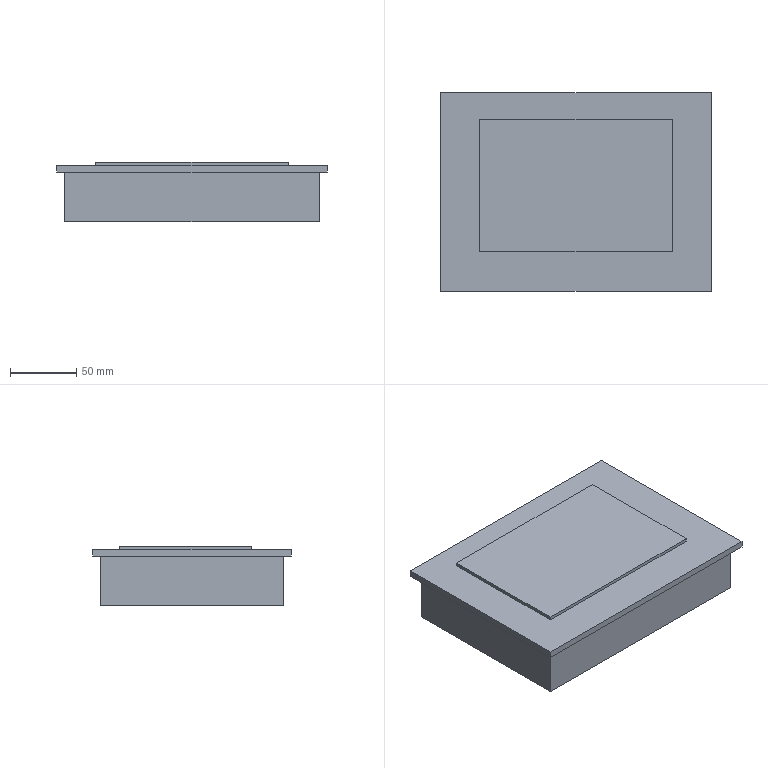Part | STEP file | 7 inch screen | 1 solid | 16 faces | box 204 x 150 x 45 mm | volume 1182850 mm3 | plane 16
STEP:
#1=CARTESIAN_POINT('',(0.,0.,0.));
#2=DIRECTION('',(0.,0.,1.));
#3=DIRECTION('',(1.,0.,0.));
#4=AXIS2_PLACEMENT_3D('',#1,#2,#3);
#5=CARTESIAN_POINT('',(102.,-75.,42.5));
#6=VERTEX_POINT('',#5);
#7=CARTESIAN_POINT('',(102.,75.,42.5));
#8=VERTEX_POINT('',#7);
#9=CARTESIAN_POINT('',(102.,-75.,42.5));
#10=DIRECTION('',(0.,1.,0.));
#11=VECTOR('',#10,1.);
#12=LINE('',#9,#11);
#13=CARTESIAN_POINT('',(0.,0.,42.5));
#14=DIRECTION('',(0.,0.,1.));
#15=DIRECTION('',(1.,0.,0.));
#16=AXIS2_PLACEMENT_3D('',#13,#14,#15);
#17=PLANE('',#16);
#18=CARTESIAN_POINT('',(102.,-75.));
#19=DIRECTION('',(0.,1.));
#20=VECTOR('',#19,1.);
#21=LINE('',#18,#20);
#22=(GEOMETRIC_REPRESENTATION_CONTEXT(2)PARAMETRIC_REPRESENTATION_CONTEXT()REPRESENTATION_CONTEXT('',''));
#23=DEFINITIONAL_REPRESENTATION('',(#21),#22);
#24=PCURVE('',#17,#23);
#25=CARTESIAN_POINT('',(102.,-75.,42.5));
#26=DIRECTION('',(-1.,0.,0.));
#27=DIRECTION('',(0.,0.,1.));
#28=AXIS2_PLACEMENT_3D('',#25,#26,#27);
#29=PLANE('',#28);
#30=CARTESIAN_POINT('',(0.,0.));
#31=DIRECTION('',(0.,1.));
#32=VECTOR('',#31,1.);
#33=LINE('',#30,#32);
#34=(GEOMETRIC_REPRESENTATION_CONTEXT(2)PARAMETRIC_REPRESENTATION_CONTEXT()REPRESENTATION_CONTEXT('',''));
#35=DEFINITIONAL_REPRESENTATION('',(#33),#34);
#36=PCURVE('',#29,#35);
#37=SURFACE_CURVE('',#12,(#24,#36),.PCURVE_S1.);
#38=EDGE_CURVE('',#6,#8,#37,.T.);
#39=ORIENTED_EDGE('',*,*,#38,.T.);
#40=CARTESIAN_POINT('',(-102.,75.,42.5));
#41=VERTEX_POINT('',#40);
#42=CARTESIAN_POINT('',(-102.,75.,42.5));
#43=DIRECTION('',(-1.,0.,0.));
#44=VECTOR('',#43,1.);
#45=LINE('',#42,#44);
#46=CARTESIAN_POINT('',(-102.,75.));
#47=DIRECTION('',(-1.,0.));
#48=VECTOR('',#47,1.);
#49=LINE('',#46,#48);
#50=(GEOMETRIC_REPRESENTATION_CONTEXT(2)PARAMETRIC_REPRESENTATION_CONTEXT()REPRESENTATION_CONTEXT('',''));
#51=DEFINITIONAL_REPRESENTATION('',(#49),#50);
#52=PCURVE('',#17,#51);
#53=CARTESIAN_POINT('',(-102.,75.,42.5));
#54=DIRECTION('',(0.,-1.,0.));
#55=DIRECTION('',(0.,0.,-1.));
#56=AXIS2_PLACEMENT_3D('',#53,#54,#55);
#57=PLANE('',#56);
#58=CARTESIAN_POINT('',(0.,0.));
#59=DIRECTION('',(0.,-1.));
#60=VECTOR('',#59,1.);
#61=LINE('',#58,#60);
#62=(GEOMETRIC_REPRESENTATION_CONTEXT(2)PARAMETRIC_REPRESENTATION_CONTEXT()REPRESENTATION_CONTEXT('',''));
#63=DEFINITIONAL_REPRESENTATION('',(#61),#62);
#64=PCURVE('',#57,#63);
#65=SURFACE_CURVE('',#45,(#52,#64),.PCURVE_S1.);
#66=EDGE_CURVE('',#8,#41,#65,.T.);
#67=ORIENTED_EDGE('',*,*,#66,.T.);
#68=CARTESIAN_POINT('',(-102.,-75.,42.5));
#69=VERTEX_POINT('',#68);
#70=CARTESIAN_POINT('',(-102.,-75.,42.5));
#71=DIRECTION('',(0.,-1.,0.));
#72=VECTOR('',#71,1.);
#73=LINE('',#70,#72);
#74=CARTESIAN_POINT('',(-102.,-75.));
#75=DIRECTION('',(0.,-1.));
#76=VECTOR('',#75,1.);
#77=LINE('',#74,#76);
#78=(GEOMETRIC_REPRESENTATION_CONTEXT(2)PARAMETRIC_REPRESENTATION_CONTEXT()REPRESENTATION_CONTEXT('',''));
#79=DEFINITIONAL_REPRESENTATION('',(#77),#78);
#80=PCURVE('',#17,#79);
#81=CARTESIAN_POINT('',(-102.,-75.,42.5));
#82=DIRECTION('',(1.,0.,0.));
#83=DIRECTION('',(0.,0.,-1.));
#84=AXIS2_PLACEMENT_3D('',#81,#82,#83);
#85=PLANE('',#84);
#86=CARTESIAN_POINT('',(0.,0.));
#87=DIRECTION('',(0.,-1.));
#88=VECTOR('',#87,1.);
#89=LINE('',#86,#88);
#90=(GEOMETRIC_REPRESENTATION_CONTEXT(2)PARAMETRIC_REPRESENTATION_CONTEXT()REPRESENTATION_CONTEXT('',''));
#91=DEFINITIONAL_REPRESENTATION('',(#89),#90);
#92=PCURVE('',#85,#91);
#93=SURFACE_CURVE('',#73,(#80,#92),.PCURVE_S1.);
#94=EDGE_CURVE('',#41,#69,#93,.T.);
#95=ORIENTED_EDGE('',*,*,#94,.T.);
#96=CARTESIAN_POINT('',(-102.,-75.,42.5));
#97=DIRECTION('',(1.,0.,0.));
#98=VECTOR('',#97,1.);
#99=LINE('',#96,#98);
#100=CARTESIAN_POINT('',(-102.,-75.));
#101=DIRECTION('',(1.,0.));
#102=VECTOR('',#101,1.);
#103=LINE('',#100,#102);
#104=(GEOMETRIC_REPRESENTATION_CONTEXT(2)PARAMETRIC_REPRESENTATION_CONTEXT()REPRESENTATION_CONTEXT('',''));
#105=DEFINITIONAL_REPRESENTATION('',(#103),#104);
#106=PCURVE('',#17,#105);
#107=CARTESIAN_POINT('',(-102.,-75.,42.5));
#108=DIRECTION('',(0.,1.,0.));
#109=DIRECTION('',(0.,0.,1.));
#110=AXIS2_PLACEMENT_3D('',#107,#108,#109);
#111=PLANE('',#110);
#112=CARTESIAN_POINT('',(0.,0.));
#113=DIRECTION('',(0.,1.));
#114=VECTOR('',#113,1.);
#115=LINE('',#112,#114);
#116=(GEOMETRIC_REPRESENTATION_CONTEXT(2)PARAMETRIC_REPRESENTATION_CONTEXT()REPRESENTATION_CONTEXT('',''));
#117=DEFINITIONAL_REPRESENTATION('',(#115),#116);
#118=PCURVE('',#111,#117);
#119=SURFACE_CURVE('',#99,(#106,#118),.PCURVE_S1.);
#120=EDGE_CURVE('',#69,#6,#119,.T.);
#121=ORIENTED_EDGE('',*,*,#120,.T.);
#122=EDGE_LOOP('',(#39,#67,#95,#121));
#123=FACE_BOUND('',#122,.T.);
#124=CARTESIAN_POINT('',(72.5,-45.,42.5));
#125=VERTEX_POINT('',#124);
#126=CARTESIAN_POINT('',(-72.5,-45.,42.5));
#127=VERTEX_POINT('',#126);
#128=CARTESIAN_POINT('',(0.,-45.,42.5));
#129=DIRECTION('',(-1.,0.,0.));
#130=VECTOR('',#129,1.);
#131=LINE('',#128,#130);
#132=CARTESIAN_POINT('',(0.,-45.));
#133=DIRECTION('',(-1.,0.));
#134=VECTOR('',#133,1.);
#135=LINE('',#132,#134);
#136=(GEOMETRIC_REPRESENTATION_CONTEXT(2)PARAMETRIC_REPRESENTATION_CONTEXT()REPRESENTATION_CONTEXT('',''));
#137=DEFINITIONAL_REPRESENTATION('',(#135),#136);
#138=PCURVE('',#17,#137);
#139=CARTESIAN_POINT('',(-72.5,-45.,45.));
#140=DIRECTION('',(0.,1.,0.));
#141=DIRECTION('',(-1.,0.,0.));
#142=AXIS2_PLACEMENT_3D('',#139,#140,#141);
#143=PLANE('',#142);
#144=CARTESIAN_POINT('',(-72.5,-2.5));
#145=DIRECTION('',(1.,0.));
#146=VECTOR('',#145,1.);
#147=LINE('',#144,#146);
#148=(GEOMETRIC_REPRESENTATION_CONTEXT(2)PARAMETRIC_REPRESENTATION_CONTEXT()REPRESENTATION_CONTEXT('',''));
#149=DEFINITIONAL_REPRESENTATION('',(#147),#148);
#150=PCURVE('',#143,#149);
#151=SURFACE_CURVE('',#131,(#138,#150),.PCURVE_S1.);
#152=EDGE_CURVE('',#125,#127,#151,.T.);
#153=ORIENTED_EDGE('',*,*,#152,.T.);
#154=CARTESIAN_POINT('',(-72.5,55.,42.5));
#155=VERTEX_POINT('',#154);
#156=CARTESIAN_POINT('',(-72.5,0.,42.5));
#157=DIRECTION('',(0.,1.,0.));
#158=VECTOR('',#157,1.);
#159=LINE('',#156,#158);
#160=CARTESIAN_POINT('',(-72.5,0.));
#161=DIRECTION('',(0.,1.));
#162=VECTOR('',#161,1.);
#163=LINE('',#160,#162);
#164=(GEOMETRIC_REPRESENTATION_CONTEXT(2)PARAMETRIC_REPRESENTATION_CONTEXT()REPRESENTATION_CONTEXT('',''));
#165=DEFINITIONAL_REPRESENTATION('',(#163),#164);
#166=PCURVE('',#17,#165);
#167=CARTESIAN_POINT('',(-72.5,55.,45.));
#168=DIRECTION('',(1.,0.,0.));
#169=DIRECTION('',(0.,0.,-1.));
#170=AXIS2_PLACEMENT_3D('',#167,#168,#169);
#171=PLANE('',#170);
#172=CARTESIAN_POINT('',(2.5,-55.));
#173=DIRECTION('',(0.,1.));
#174=VECTOR('',#173,1.);
#175=LINE('',#172,#174);
#176=(GEOMETRIC_REPRESENTATION_CONTEXT(2)PARAMETRIC_REPRESENTATION_CONTEXT()REPRESENTATION_CONTEXT('',''));
#177=DEFINITIONAL_REPRESENTATION('',(#175),#176);
#178=PCURVE('',#171,#177);
#179=SURFACE_CURVE('',#159,(#166,#178),.PCURVE_S1.);
#180=EDGE_CURVE('',#127,#155,#179,.T.);
#181=ORIENTED_EDGE('',*,*,#180,.T.);
#182=CARTESIAN_POINT('',(72.5,55.,42.5));
#183=VERTEX_POINT('',#182);
#184=CARTESIAN_POINT('',(0.,55.,42.5));
#185=DIRECTION('',(1.,0.,0.));
#186=VECTOR('',#185,1.);
#187=LINE('',#184,#186);
#188=CARTESIAN_POINT('',(0.,55.));
#189=DIRECTION('',(1.,0.));
#190=VECTOR('',#189,1.);
#191=LINE('',#188,#190);
#192=(GEOMETRIC_REPRESENTATION_CONTEXT(2)PARAMETRIC_REPRESENTATION_CONTEXT()REPRESENTATION_CONTEXT('',''));
#193=DEFINITIONAL_REPRESENTATION('',(#191),#192);
#194=PCURVE('',#17,#193);
#195=CARTESIAN_POINT('',(-72.5,55.,45.));
#196=DIRECTION('',(0.,-1.,0.));
#197=DIRECTION('',(1.,0.,0.));
#198=AXIS2_PLACEMENT_3D('',#195,#196,#197);
#199=PLANE('',#198);
#200=CARTESIAN_POINT('',(72.5,-2.5));
#201=DIRECTION('',(1.,0.));
#202=VECTOR('',#201,1.);
#203=LINE('',#200,#202);
#204=(GEOMETRIC_REPRESENTATION_CONTEXT(2)PARAMETRIC_REPRESENTATION_CONTEXT()REPRESENTATION_CONTEXT('',''));
#205=DEFINITIONAL_REPRESENTATION('',(#203),#204);
#206=PCURVE('',#199,#205);
#207=SURFACE_CURVE('',#187,(#194,#206),.PCURVE_S1.);
#208=EDGE_CURVE('',#155,#183,#207,.T.);
#209=ORIENTED_EDGE('',*,*,#208,.T.);
#210=CARTESIAN_POINT('',(72.5,0.,42.5));
#211=DIRECTION('',(0.,-1.,0.));
#212=VECTOR('',#211,1.);
#213=LINE('',#210,#212);
#214=CARTESIAN_POINT('',(72.5,0.));
#215=DIRECTION('',(0.,-1.));
#216=VECTOR('',#215,1.);
#217=LINE('',#214,#216);
#218=(GEOMETRIC_REPRESENTATION_CONTEXT(2)PARAMETRIC_REPRESENTATION_CONTEXT()REPRESENTATION_CONTEXT('',''));
#219=DEFINITIONAL_REPRESENTATION('',(#217),#218);
#220=PCURVE('',#17,#219);
#221=CARTESIAN_POINT('',(72.5,55.,45.));
#222=DIRECTION('',(-1.,0.,0.));
#223=DIRECTION('',(0.,-1.,0.));
#224=AXIS2_PLACEMENT_3D('',#221,#222,#223);
#225=PLANE('',#224);
#226=CARTESIAN_POINT('',(55.,-2.5));
#227=DIRECTION('',(1.,0.));
#228=VECTOR('',#227,1.);
#229=LINE('',#226,#228);
#230=(GEOMETRIC_REPRESENTATION_CONTEXT(2)PARAMETRIC_REPRESENTATION_CONTEXT()REPRESENTATION_CONTEXT('',''));
#231=DEFINITIONAL_REPRESENTATION('',(#229),#230);
#232=PCURVE('',#225,#231);
#233=SURFACE_CURVE('',#213,(#220,#232),.PCURVE_S1.);
#234=EDGE_CURVE('',#183,#125,#233,.T.);
#235=ORIENTED_EDGE('',*,*,#234,.T.);
#236=EDGE_LOOP('',(#153,#181,#209,#235));
#237=FACE_BOUND('',#236,.T.);
#238=ADVANCED_FACE('',(#123,#237),#17,.T.);
#239=CARTESIAN_POINT('',(96.,-69.,37.5));
#240=VERTEX_POINT('',#239);
#241=CARTESIAN_POINT('',(96.,69.,37.5));
#242=VERTEX_POINT('',#241);
#243=CARTESIAN_POINT('',(96.,-69.,37.5));
#244=DIRECTION('',(0.,1.,0.));
#245=VECTOR('',#244,1.);
#246=LINE('',#243,#245);
#247=CARTESIAN_POINT('',(96.,-69.,40.));
#248=DIRECTION('',(-1.,0.,0.));
#249=DIRECTION('',(0.,0.,1.));
#250=AXIS2_PLACEMENT_3D('',#247,#248,#249);
#251=PLANE('',#250);
#252=CARTESIAN_POINT('',(-2.5,0.));
#253=DIRECTION('',(0.,1.));
#254=VECTOR('',#253,1.);
#255=LINE('',#252,#254);
#256=(GEOMETRIC_REPRESENTATION_CONTEXT(2)PARAMETRIC_REPRESENTATION_CONTEXT()REPRESENTATION_CONTEXT('',''));
#257=DEFINITIONAL_REPRESENTATION('',(#255),#256);
#258=PCURVE('',#251,#257);
#259=CARTESIAN_POINT('',(0.,0.,37.5));
#260=DIRECTION('',(0.,0.,1.));
#261=DIRECTION('',(1.,0.,0.));
#262=AXIS2_PLACEMENT_3D('',#259,#260,#261);
#263=PLANE('',#262);
#264=CARTESIAN_POINT('',(96.,-69.));
#265=DIRECTION('',(0.,1.));
#266=VECTOR('',#265,1.);
#267=LINE('',#264,#266);
#268=(GEOMETRIC_REPRESENTATION_CONTEXT(2)PARAMETRIC_REPRESENTATION_CONTEXT()REPRESENTATION_CONTEXT('',''));
#269=DEFINITIONAL_REPRESENTATION('',(#267),#268);
#270=PCURVE('',#263,#269);
#271=SURFACE_CURVE('',#246,(#258,#270),.PCURVE_S1.);
#272=EDGE_CURVE('',#240,#242,#271,.T.);
#273=ORIENTED_EDGE('',*,*,#272,.F.);
#274=CARTESIAN_POINT('',(96.,-69.,0.));
#275=VERTEX_POINT('',#274);
#276=CARTESIAN_POINT('',(96.,-69.,40.));
#277=DIRECTION('',(0.,0.,-1.));
#278=VECTOR('',#277,1.);
#279=LINE('',#276,#278);
#280=CARTESIAN_POINT('',(0.,0.));
#281=DIRECTION('',(-1.,0.));
#282=VECTOR('',#281,1.);
#283=LINE('',#280,#282);
#284=(GEOMETRIC_REPRESENTATION_CONTEXT(2)PARAMETRIC_REPRESENTATION_CONTEXT()REPRESENTATION_CONTEXT('',''));
#285=DEFINITIONAL_REPRESENTATION('',(#283),#284);
#286=PCURVE('',#251,#285);
#287=CARTESIAN_POINT('',(-96.,-69.,40.));
#288=DIRECTION('',(0.,1.,0.));
#289=DIRECTION('',(0.,0.,1.));
#290=AXIS2_PLACEMENT_3D('',#287,#288,#289);
#291=PLANE('',#290);
#292=CARTESIAN_POINT('',(0.,192.));
#293=DIRECTION('',(-1.,0.));
#294=VECTOR('',#293,1.);
#295=LINE('',#292,#294);
#296=(GEOMETRIC_REPRESENTATION_CONTEXT(2)PARAMETRIC_REPRESENTATION_CONTEXT()REPRESENTATION_CONTEXT('',''));
#297=DEFINITIONAL_REPRESENTATION('',(#295),#296);
#298=PCURVE('',#291,#297);
#299=SURFACE_CURVE('',#279,(#286,#298),.PCURVE_S1.);
#300=EDGE_CURVE('',#240,#275,#299,.T.);
#301=ORIENTED_EDGE('',*,*,#300,.T.);
#302=CARTESIAN_POINT('',(96.,69.,0.));
#303=VERTEX_POINT('',#302);
#304=CARTESIAN_POINT('',(96.,-69.,0.));
#305=DIRECTION('',(0.,1.,0.));
#306=VECTOR('',#305,1.);
#307=LINE('',#304,#306);
#308=CARTESIAN_POINT('',(-40.,0.));
#309=DIRECTION('',(0.,1.));
#310=VECTOR('',#309,1.);
#311=LINE('',#308,#310);
#312=(GEOMETRIC_REPRESENTATION_CONTEXT(2)PARAMETRIC_REPRESENTATION_CONTEXT()REPRESENTATION_CONTEXT('',''));
#313=DEFINITIONAL_REPRESENTATION('',(#311),#312);
#314=PCURVE('',#251,#313);
#315=CARTESIAN_POINT('',(0.,0.,0.));
#316=DIRECTION('',(0.,0.,-1.));
#317=DIRECTION('',(-1.,0.,0.));
#318=AXIS2_PLACEMENT_3D('',#315,#316,#317);
#319=PLANE('',#318);
#320=CARTESIAN_POINT('',(-96.,-69.));
#321=DIRECTION('',(0.,1.));
#322=VECTOR('',#321,1.);
#323=LINE('',#320,#322);
#324=(GEOMETRIC_REPRESENTATION_CONTEXT(2)PARAMETRIC_REPRESENTATION_CONTEXT()REPRESENTATION_CONTEXT('',''));
#325=DEFINITIONAL_REPRESENTATION('',(#323),#324);
#326=PCURVE('',#319,#325);
#327=SURFACE_CURVE('',#307,(#314,#326),.PCURVE_S1.);
#328=EDGE_CURVE('',#275,#303,#327,.T.);
#329=ORIENTED_EDGE('',*,*,#328,.T.);
#330=CARTESIAN_POINT('',(96.,69.,40.));
#331=DIRECTION('',(0.,0.,-1.));
#332=VECTOR('',#331,1.);
#333=LINE('',#330,#332);
#334=CARTESIAN_POINT('',(0.,138.));
#335=DIRECTION('',(-1.,0.));
#336=VECTOR('',#335,1.);
#337=LINE('',#334,#336);
#338=(GEOMETRIC_REPRESENTATION_CONTEXT(2)PARAMETRIC_REPRESENTATION_CONTEXT()REPRESENTATION_CONTEXT('',''));
#339=DEFINITIONAL_REPRESENTATION('',(#337),#338);
#340=PCURVE('',#251,#339);
#341=CARTESIAN_POINT('',(-96.,69.,40.));
#342=DIRECTION('',(0.,-1.,0.));
#343=DIRECTION('',(0.,0.,-1.));
#344=AXIS2_PLACEMENT_3D('',#341,#342,#343);
#345=PLANE('',#344);
#346=CARTESIAN_POINT('',(0.,192.));
#347=DIRECTION('',(1.,0.));
#348=VECTOR('',#347,1.);
#349=LINE('',#346,#348);
#350=(GEOMETRIC_REPRESENTATION_CONTEXT(2)PARAMETRIC_REPRESENTATION_CONTEXT()REPRESENTATION_CONTEXT('',''));
#351=DEFINITIONAL_REPRESENTATION('',(#349),#350);
#352=PCURVE('',#345,#351);
#353=SURFACE_CURVE('',#333,(#340,#352),.PCURVE_S1.);
#354=EDGE_CURVE('',#242,#303,#353,.T.);
#355=ORIENTED_EDGE('',*,*,#354,.F.);
#356=EDGE_LOOP('',(#273,#301,#329,#355));
#357=FACE_BOUND('',#356,.T.);
#358=ADVANCED_FACE('',(#357),#251,.F.);
#359=CARTESIAN_POINT('',(-96.,69.,37.5));
#360=VERTEX_POINT('',#359);
#361=CARTESIAN_POINT('',(-96.,69.,37.5));
#362=DIRECTION('',(-1.,0.,0.));
#363=VECTOR('',#362,1.);
#364=LINE('',#361,#363);
#365=CARTESIAN_POINT('',(2.5,0.));
#366=DIRECTION('',(0.,-1.));
#367=VECTOR('',#366,1.);
#368=LINE('',#365,#367);
#369=(GEOMETRIC_REPRESENTATION_CONTEXT(2)PARAMETRIC_REPRESENTATION_CONTEXT()REPRESENTATION_CONTEXT('',''));
#370=DEFINITIONAL_REPRESENTATION('',(#368),#369);
#371=PCURVE('',#345,#370);
#372=CARTESIAN_POINT('',(-96.,69.));
#373=DIRECTION('',(-1.,0.));
#374=VECTOR('',#373,1.);
#375=LINE('',#372,#374);
#376=(GEOMETRIC_REPRESENTATION_CONTEXT(2)PARAMETRIC_REPRESENTATION_CONTEXT()REPRESENTATION_CONTEXT('',''));
#377=DEFINITIONAL_REPRESENTATION('',(#375),#376);
#378=PCURVE('',#263,#377);
#379=SURFACE_CURVE('',#364,(#371,#378),.PCURVE_S1.);
#380=EDGE_CURVE('',#242,#360,#379,.T.);
#381=ORIENTED_EDGE('',*,*,#380,.F.);
#382=ORIENTED_EDGE('',*,*,#354,.T.);
#383=CARTESIAN_POINT('',(-96.,69.,0.));
#384=VERTEX_POINT('',#383);
#385=CARTESIAN_POINT('',(-96.,69.,0.));
#386=DIRECTION('',(-1.,0.,0.));
#387=VECTOR('',#386,1.);
#388=LINE('',#385,#387);
#389=CARTESIAN_POINT('',(40.,0.));
#390=DIRECTION('',(0.,-1.));
#391=VECTOR('',#390,1.);
#392=LINE('',#389,#391);
#393=(GEOMETRIC_REPRESENTATION_CONTEXT(2)PARAMETRIC_REPRESENTATION_CONTEXT()REPRESENTATION_CONTEXT('',''));
#394=DEFINITIONAL_REPRESENTATION('',(#392),#393);
#395=PCURVE('',#345,#394);
#396=CARTESIAN_POINT('',(96.,69.));
#397=DIRECTION('',(1.,0.));
#398=VECTOR('',#397,1.);
#399=LINE('',#396,#398);
#400=(GEOMETRIC_REPRESENTATION_CONTEXT(2)PARAMETRIC_REPRESENTATION_CONTEXT()REPRESENTATION_CONTEXT('',''));
#401=DEFINITIONAL_REPRESENTATION('',(#399),#400);
#402=PCURVE('',#319,#401);
#403=SURFACE_CURVE('',#388,(#395,#402),.PCURVE_S1.);
#404=EDGE_CURVE('',#303,#384,#403,.T.);
#405=ORIENTED_EDGE('',*,*,#404,.T.);
#406=CARTESIAN_POINT('',(-96.,69.,40.));
#407=DIRECTION('',(0.,0.,-1.));
#408=VECTOR('',#407,1.);
#409=LINE('',#406,#408);
#410=CARTESIAN_POINT('',(0.,0.));
#411=DIRECTION('',(1.,0.));
#412=VECTOR('',#411,1.);
#413=LINE('',#410,#412);
#414=(GEOMETRIC_REPRESENTATION_CONTEXT(2)PARAMETRIC_REPRESENTATION_CONTEXT()REPRESENTATION_CONTEXT('',''));
#415=DEFINITIONAL_REPRESENTATION('',(#413),#414);
#416=PCURVE('',#345,#415);
#417=CARTESIAN_POINT('',(-96.,-69.,40.));
#418=DIRECTION('',(1.,0.,0.));
#419=DIRECTION('',(0.,0.,-1.));
#420=AXIS2_PLACEMENT_3D('',#417,#418,#419);
#421=PLANE('',#420);
#422=CARTESIAN_POINT('',(0.,138.));
#423=DIRECTION('',(1.,0.));
#424=VECTOR('',#423,1.);
#425=LINE('',#422,#424);
#426=(GEOMETRIC_REPRESENTATION_CONTEXT(2)PARAMETRIC_REPRESENTATION_CONTEXT()REPRESENTATION_CONTEXT('',''));
#427=DEFINITIONAL_REPRESENTATION('',(#425),#426);
#428=PCURVE('',#421,#427);
#429=SURFACE_CURVE('',#409,(#416,#428),.PCURVE_S1.);
#430=EDGE_CURVE('',#360,#384,#429,.T.);
#431=ORIENTED_EDGE('',*,*,#430,.F.);
#432=EDGE_LOOP('',(#381,#382,#405,#431));
#433=FACE_BOUND('',#432,.T.);
#434=ADVANCED_FACE('',(#433),#345,.F.);
#435=CARTESIAN_POINT('',(-96.,-69.,37.5));
#436=VERTEX_POINT('',#435);
#437=CARTESIAN_POINT('',(-96.,-69.,37.5));
#438=DIRECTION('',(0.,-1.,0.));
#439=VECTOR('',#438,1.);
#440=LINE('',#437,#439);
#441=CARTESIAN_POINT('',(2.5,0.));
#442=DIRECTION('',(0.,-1.));
#443=VECTOR('',#442,1.);
#444=LINE('',#441,#443);
#445=(GEOMETRIC_REPRESENTATION_CONTEXT(2)PARAMETRIC_REPRESENTATION_CONTEXT()REPRESENTATION_CONTEXT('',''));
#446=DEFINITIONAL_REPRESENTATION('',(#444),#445);
#447=PCURVE('',#421,#446);
#448=CARTESIAN_POINT('',(-96.,-69.));
#449=DIRECTION('',(0.,-1.));
#450=VECTOR('',#449,1.);
#451=LINE('',#448,#450);
#452=(GEOMETRIC_REPRESENTATION_CONTEXT(2)PARAMETRIC_REPRESENTATION_CONTEXT()REPRESENTATION_CONTEXT('',''));
#453=DEFINITIONAL_REPRESENTATION('',(#451),#452);
#454=PCURVE('',#263,#453);
#455=SURFACE_CURVE('',#440,(#447,#454),.PCURVE_S1.);
#456=EDGE_CURVE('',#360,#436,#455,.T.);
#457=ORIENTED_EDGE('',*,*,#456,.F.);
#458=ORIENTED_EDGE('',*,*,#430,.T.);
#459=CARTESIAN_POINT('',(-96.,-69.,0.));
#460=VERTEX_POINT('',#459);
#461=CARTESIAN_POINT('',(-96.,-69.,0.));
#462=DIRECTION('',(0.,-1.,0.));
#463=VECTOR('',#462,1.);
#464=LINE('',#461,#463);
#465=CARTESIAN_POINT('',(40.,0.));
#466=DIRECTION('',(0.,-1.));
#467=VECTOR('',#466,1.);
#468=LINE('',#465,#467);
#469=(GEOMETRIC_REPRESENTATION_CONTEXT(2)PARAMETRIC_REPRESENTATION_CONTEXT()REPRESENTATION_CONTEXT('',''));
#470=DEFINITIONAL_REPRESENTATION('',(#468),#469);
#471=PCURVE('',#421,#470);
#472=CARTESIAN_POINT('',(96.,-69.));
#473=DIRECTION('',(0.,-1.));
#474=VECTOR('',#473,1.);
#475=LINE('',#472,#474);
#476=(GEOMETRIC_REPRESENTATION_CONTEXT(2)PARAMETRIC_REPRESENTATION_CONTEXT()REPRESENTATION_CONTEXT('',''));
#477=DEFINITIONAL_REPRESENTATION('',(#475),#476);
#478=PCURVE('',#319,#477);
#479=SURFACE_CURVE('',#464,(#471,#478),.PCURVE_S1.);
#480=EDGE_CURVE('',#384,#460,#479,.T.);
#481=ORIENTED_EDGE('',*,*,#480,.T.);
#482=CARTESIAN_POINT('',(-96.,-69.,40.));
#483=DIRECTION('',(0.,0.,-1.));
#484=VECTOR('',#483,1.);
#485=LINE('',#482,#484);
#486=CARTESIAN_POINT('',(0.,0.));
#487=DIRECTION('',(1.,0.));
#488=VECTOR('',#487,1.);
#489=LINE('',#486,#488);
#490=(GEOMETRIC_REPRESENTATION_CONTEXT(2)PARAMETRIC_REPRESENTATION_CONTEXT()REPRESENTATION_CONTEXT('',''));
#491=DEFINITIONAL_REPRESENTATION('',(#489),#490);
#492=PCURVE('',#421,#491);
#493=CARTESIAN_POINT('',(0.,0.));
#494=DIRECTION('',(-1.,0.));
#495=VECTOR('',#494,1.);
#496=LINE('',#493,#495);
#497=(GEOMETRIC_REPRESENTATION_CONTEXT(2)PARAMETRIC_REPRESENTATION_CONTEXT()REPRESENTATION_CONTEXT('',''));
#498=DEFINITIONAL_REPRESENTATION('',(#496),#497);
#499=PCURVE('',#291,#498);
#500=SURFACE_CURVE('',#485,(#492,#499),.PCURVE_S1.);
#501=EDGE_CURVE('',#436,#460,#500,.T.);
#502=ORIENTED_EDGE('',*,*,#501,.F.);
#503=EDGE_LOOP('',(#457,#458,#481,#502));
#504=FACE_BOUND('',#503,.T.);
#505=ADVANCED_FACE('',(#504),#421,.F.);
#506=CARTESIAN_POINT('',(-96.,-69.,37.5));
#507=DIRECTION('',(1.,0.,0.));
#508=VECTOR('',#507,1.);
#509=LINE('',#506,#508);
#510=CARTESIAN_POINT('',(-2.5,0.));
#511=DIRECTION('',(0.,1.));
#512=VECTOR('',#511,1.);
#513=LINE('',#510,#512);
#514=(GEOMETRIC_REPRESENTATION_CONTEXT(2)PARAMETRIC_REPRESENTATION_CONTEXT()REPRESENTATION_CONTEXT('',''));
#515=DEFINITIONAL_REPRESENTATION('',(#513),#514);
#516=PCURVE('',#291,#515);
#517=CARTESIAN_POINT('',(-96.,-69.));
#518=DIRECTION('',(1.,0.));
#519=VECTOR('',#518,1.);
#520=LINE('',#517,#519);
#521=(GEOMETRIC_REPRESENTATION_CONTEXT(2)PARAMETRIC_REPRESENTATION_CONTEXT()REPRESENTATION_CONTEXT('',''));
#522=DEFINITIONAL_REPRESENTATION('',(#520),#521);
#523=PCURVE('',#263,#522);
#524=SURFACE_CURVE('',#509,(#516,#523),.PCURVE_S1.);
#525=EDGE_CURVE('',#436,#240,#524,.T.);
#526=ORIENTED_EDGE('',*,*,#525,.F.);
#527=ORIENTED_EDGE('',*,*,#501,.T.);
#528=CARTESIAN_POINT('',(-96.,-69.,0.));
#529=DIRECTION('',(1.,0.,0.));
#530=VECTOR('',#529,1.);
#531=LINE('',#528,#530);
#532=CARTESIAN_POINT('',(-40.,0.));
#533=DIRECTION('',(0.,1.));
#534=VECTOR('',#533,1.);
#535=LINE('',#532,#534);
#536=(GEOMETRIC_REPRESENTATION_CONTEXT(2)PARAMETRIC_REPRESENTATION_CONTEXT()REPRESENTATION_CONTEXT('',''));
#537=DEFINITIONAL_REPRESENTATION('',(#535),#536);
#538=PCURVE('',#291,#537);
#539=CARTESIAN_POINT('',(96.,-69.));
#540=DIRECTION('',(-1.,0.));
#541=VECTOR('',#540,1.);
#542=LINE('',#539,#541);
#543=(GEOMETRIC_REPRESENTATION_CONTEXT(2)PARAMETRIC_REPRESENTATION_CONTEXT()REPRESENTATION_CONTEXT('',''));
#544=DEFINITIONAL_REPRESENTATION('',(#542),#543);
#545=PCURVE('',#319,#544);
#546=SURFACE_CURVE('',#531,(#538,#545),.PCURVE_S1.);
#547=EDGE_CURVE('',#460,#275,#546,.T.);
#548=ORIENTED_EDGE('',*,*,#547,.T.);
#549=ORIENTED_EDGE('',*,*,#300,.F.);
#550=EDGE_LOOP('',(#526,#527,#548,#549));
#551=FACE_BOUND('',#550,.T.);
#552=ADVANCED_FACE('',(#551),#291,.F.);
#553=ORIENTED_EDGE('',*,*,#328,.F.);
#554=ORIENTED_EDGE('',*,*,#547,.F.);
#555=ORIENTED_EDGE('',*,*,#480,.F.);
#556=ORIENTED_EDGE('',*,*,#404,.F.);
#557=EDGE_LOOP('',(#553,#554,#555,#556));
#558=FACE_BOUND('',#557,.T.);
#559=ADVANCED_FACE('',(#558),#319,.T.);
#560=CARTESIAN_POINT('',(102.,-75.,37.5));
#561=VERTEX_POINT('',#560);
#562=CARTESIAN_POINT('',(102.,75.,37.5));
#563=VERTEX_POINT('',#562);
#564=CARTESIAN_POINT('',(102.,-75.,37.5));
#565=DIRECTION('',(0.,1.,0.));
#566=VECTOR('',#565,1.);
#567=LINE('',#564,#566);
#568=CARTESIAN_POINT('',(102.,-75.));
#569=DIRECTION('',(0.,1.));
#570=VECTOR('',#569,1.);
#571=LINE('',#568,#570);
#572=(GEOMETRIC_REPRESENTATION_CONTEXT(2)PARAMETRIC_REPRESENTATION_CONTEXT()REPRESENTATION_CONTEXT('',''));
#573=DEFINITIONAL_REPRESENTATION('',(#571),#572);
#574=PCURVE('',#263,#573);
#575=CARTESIAN_POINT('',(-5.,0.));
#576=DIRECTION('',(0.,1.));
#577=VECTOR('',#576,1.);
#578=LINE('',#575,#577);
#579=(GEOMETRIC_REPRESENTATION_CONTEXT(2)PARAMETRIC_REPRESENTATION_CONTEXT()REPRESENTATION_CONTEXT('',''));
#580=DEFINITIONAL_REPRESENTATION('',(#578),#579);
#581=PCURVE('',#29,#580);
#582=SURFACE_CURVE('',#567,(#574,#581),.PCURVE_S1.);
#583=EDGE_CURVE('',#561,#563,#582,.T.);
#584=ORIENTED_EDGE('',*,*,#583,.F.);
#585=CARTESIAN_POINT('',(-102.,-75.,37.5));
#586=VERTEX_POINT('',#585);
#587=CARTESIAN_POINT('',(-102.,-75.,37.5));
#588=DIRECTION('',(1.,0.,0.));
#589=VECTOR('',#588,1.);
#590=LINE('',#587,#589);
#591=CARTESIAN_POINT('',(-102.,-75.));
#592=DIRECTION('',(1.,0.));
#593=VECTOR('',#592,1.);
#594=LINE('',#591,#593);
#595=(GEOMETRIC_REPRESENTATION_CONTEXT(2)PARAMETRIC_REPRESENTATION_CONTEXT()REPRESENTATION_CONTEXT('',''));
#596=DEFINITIONAL_REPRESENTATION('',(#594),#595);
#597=PCURVE('',#263,#596);
#598=CARTESIAN_POINT('',(-5.,0.));
#599=DIRECTION('',(0.,1.));
#600=VECTOR('',#599,1.);
#601=LINE('',#598,#600);
#602=(GEOMETRIC_REPRESENTATION_CONTEXT(2)PARAMETRIC_REPRESENTATION_CONTEXT()REPRESENTATION_CONTEXT('',''));
#603=DEFINITIONAL_REPRESENTATION('',(#601),#602);
#604=PCURVE('',#111,#603);
#605=SURFACE_CURVE('',#590,(#597,#604),.PCURVE_S1.);
#606=EDGE_CURVE('',#586,#561,#605,.T.);
#607=ORIENTED_EDGE('',*,*,#606,.F.);
#608=CARTESIAN_POINT('',(-102.,75.,37.5));
#609=VERTEX_POINT('',#608);
#610=CARTESIAN_POINT('',(-102.,-75.,37.5));
#611=DIRECTION('',(0.,-1.,0.));
#612=VECTOR('',#611,1.);
#613=LINE('',#610,#612);
#614=CARTESIAN_POINT('',(-102.,-75.));
#615=DIRECTION('',(0.,-1.));
#616=VECTOR('',#615,1.);
#617=LINE('',#614,#616);
#618=(GEOMETRIC_REPRESENTATION_CONTEXT(2)PARAMETRIC_REPRESENTATION_CONTEXT()REPRESENTATION_CONTEXT('',''));
#619=DEFINITIONAL_REPRESENTATION('',(#617),#618);
#620=PCURVE('',#263,#619);
#621=CARTESIAN_POINT('',(5.,0.));
#622=DIRECTION('',(0.,-1.));
#623=VECTOR('',#622,1.);
#624=LINE('',#621,#623);
#625=(GEOMETRIC_REPRESENTATION_CONTEXT(2)PARAMETRIC_REPRESENTATION_CONTEXT()REPRESENTATION_CONTEXT('',''));
#626=DEFINITIONAL_REPRESENTATION('',(#624),#625);
#627=PCURVE('',#85,#626);
#628=SURFACE_CURVE('',#613,(#620,#627),.PCURVE_S1.);
#629=EDGE_CURVE('',#609,#586,#628,.T.);
#630=ORIENTED_EDGE('',*,*,#629,.F.);
#631=CARTESIAN_POINT('',(-102.,75.,37.5));
#632=DIRECTION('',(-1.,0.,0.));
#633=VECTOR('',#632,1.);
#634=LINE('',#631,#633);
#635=CARTESIAN_POINT('',(-102.,75.));
#636=DIRECTION('',(-1.,0.));
#637=VECTOR('',#636,1.);
#638=LINE('',#635,#637);
#639=(GEOMETRIC_REPRESENTATION_CONTEXT(2)PARAMETRIC_REPRESENTATION_CONTEXT()REPRESENTATION_CONTEXT('',''));
#640=DEFINITIONAL_REPRESENTATION('',(#638),#639);
#641=PCURVE('',#263,#640);
#642=CARTESIAN_POINT('',(5.,0.));
#643=DIRECTION('',(0.,-1.));
#644=VECTOR('',#643,1.);
#645=LINE('',#642,#644);
#646=(GEOMETRIC_REPRESENTATION_CONTEXT(2)PARAMETRIC_REPRESENTATION_CONTEXT()REPRESENTATION_CONTEXT('',''));
#647=DEFINITIONAL_REPRESENTATION('',(#645),#646);
#648=PCURVE('',#57,#647);
#649=SURFACE_CURVE('',#634,(#641,#648),.PCURVE_S1.);
#650=EDGE_CURVE('',#563,#609,#649,.T.);
#651=ORIENTED_EDGE('',*,*,#650,.F.);
#652=EDGE_LOOP('',(#584,#607,#630,#651));
#653=FACE_BOUND('',#652,.T.);
#654=ORIENTED_EDGE('',*,*,#525,.T.);
#655=ORIENTED_EDGE('',*,*,#272,.T.);
#656=ORIENTED_EDGE('',*,*,#380,.T.);
#657=ORIENTED_EDGE('',*,*,#456,.T.);
#658=EDGE_LOOP('',(#654,#655,#656,#657));
#659=FACE_BOUND('',#658,.T.);
#660=ADVANCED_FACE('',(#653,#659),#263,.F.);
#661=ORIENTED_EDGE('',*,*,#583,.T.);
#662=CARTESIAN_POINT('',(102.,75.,42.5));
#663=DIRECTION('',(0.,0.,-1.));
#664=VECTOR('',#663,1.);
#665=LINE('',#662,#664);
#666=CARTESIAN_POINT('',(0.,150.));
#667=DIRECTION('',(-1.,0.));
#668=VECTOR('',#667,1.);
#669=LINE('',#666,#668);
#670=(GEOMETRIC_REPRESENTATION_CONTEXT(2)PARAMETRIC_REPRESENTATION_CONTEXT()REPRESENTATION_CONTEXT('',''));
#671=DEFINITIONAL_REPRESENTATION('',(#669),#670);
#672=PCURVE('',#29,#671);
#673=CARTESIAN_POINT('',(0.,204.));
#674=DIRECTION('',(1.,0.));
#675=VECTOR('',#674,1.);
#676=LINE('',#673,#675);
#677=(GEOMETRIC_REPRESENTATION_CONTEXT(2)PARAMETRIC_REPRESENTATION_CONTEXT()REPRESENTATION_CONTEXT('',''));
#678=DEFINITIONAL_REPRESENTATION('',(#676),#677);
#679=PCURVE('',#57,#678);
#680=SURFACE_CURVE('',#665,(#672,#679),.PCURVE_S1.);
#681=EDGE_CURVE('',#8,#563,#680,.T.);
#682=ORIENTED_EDGE('',*,*,#681,.F.);
#683=ORIENTED_EDGE('',*,*,#38,.F.);
#684=CARTESIAN_POINT('',(102.,-75.,42.5));
#685=DIRECTION('',(0.,0.,-1.));
#686=VECTOR('',#685,1.);
#687=LINE('',#684,#686);
#688=CARTESIAN_POINT('',(0.,0.));
#689=DIRECTION('',(-1.,0.));
#690=VECTOR('',#689,1.);
#691=LINE('',#688,#690);
#692=(GEOMETRIC_REPRESENTATION_CONTEXT(2)PARAMETRIC_REPRESENTATION_CONTEXT()REPRESENTATION_CONTEXT('',''));
#693=DEFINITIONAL_REPRESENTATION('',(#691),#692);
#694=PCURVE('',#29,#693);
#695=CARTESIAN_POINT('',(0.,204.));
#696=DIRECTION('',(-1.,0.));
#697=VECTOR('',#696,1.);
#698=LINE('',#695,#697);
#699=(GEOMETRIC_REPRESENTATION_CONTEXT(2)PARAMETRIC_REPRESENTATION_CONTEXT()REPRESENTATION_CONTEXT('',''));
#700=DEFINITIONAL_REPRESENTATION('',(#698),#699);
#701=PCURVE('',#111,#700);
#702=SURFACE_CURVE('',#687,(#694,#701),.PCURVE_S1.);
#703=EDGE_CURVE('',#6,#561,#702,.T.);
#704=ORIENTED_EDGE('',*,*,#703,.T.);
#705=EDGE_LOOP('',(#661,#682,#683,#704));
#706=FACE_BOUND('',#705,.T.);
#707=ADVANCED_FACE('',(#706),#29,.F.);
#708=ORIENTED_EDGE('',*,*,#650,.T.);
#709=CARTESIAN_POINT('',(-102.,75.,42.5));
#710=DIRECTION('',(0.,0.,-1.));
#711=VECTOR('',#710,1.);
#712=LINE('',#709,#711);
#713=CARTESIAN_POINT('',(0.,0.));
#714=DIRECTION('',(1.,0.));
#715=VECTOR('',#714,1.);
#716=LINE('',#713,#715);
#717=(GEOMETRIC_REPRESENTATION_CONTEXT(2)PARAMETRIC_REPRESENTATION_CONTEXT()REPRESENTATION_CONTEXT('',''));
#718=DEFINITIONAL_REPRESENTATION('',(#716),#717);
#719=PCURVE('',#57,#718);
#720=CARTESIAN_POINT('',(0.,150.));
#721=DIRECTION('',(1.,0.));
#722=VECTOR('',#721,1.);
#723=LINE('',#720,#722);
#724=(GEOMETRIC_REPRESENTATION_CONTEXT(2)PARAMETRIC_REPRESENTATION_CONTEXT()REPRESENTATION_CONTEXT('',''));
#725=DEFINITIONAL_REPRESENTATION('',(#723),#724);
#726=PCURVE('',#85,#725);
#727=SURFACE_CURVE('',#712,(#719,#726),.PCURVE_S1.);
#728=EDGE_CURVE('',#41,#609,#727,.T.);
#729=ORIENTED_EDGE('',*,*,#728,.F.);
#730=ORIENTED_EDGE('',*,*,#66,.F.);
#731=ORIENTED_EDGE('',*,*,#681,.T.);
#732=EDGE_LOOP('',(#708,#729,#730,#731));
#733=FACE_BOUND('',#732,.T.);
#734=ADVANCED_FACE('',(#733),#57,.F.);
#735=ORIENTED_EDGE('',*,*,#629,.T.);
#736=CARTESIAN_POINT('',(-102.,-75.,42.5));
#737=DIRECTION('',(0.,0.,-1.));
#738=VECTOR('',#737,1.);
#739=LINE('',#736,#738);
#740=CARTESIAN_POINT('',(0.,0.));
#741=DIRECTION('',(1.,0.));
#742=VECTOR('',#741,1.);
#743=LINE('',#740,#742);
#744=(GEOMETRIC_REPRESENTATION_CONTEXT(2)PARAMETRIC_REPRESENTATION_CONTEXT()REPRESENTATION_CONTEXT('',''));
#745=DEFINITIONAL_REPRESENTATION('',(#743),#744);
#746=PCURVE('',#85,#745);
#747=CARTESIAN_POINT('',(0.,0.));
#748=DIRECTION('',(-1.,0.));
#749=VECTOR('',#748,1.);
#750=LINE('',#747,#749);
#751=(GEOMETRIC_REPRESENTATION_CONTEXT(2)PARAMETRIC_REPRESENTATION_CONTEXT()REPRESENTATION_CONTEXT('',''));
#752=DEFINITIONAL_REPRESENTATION('',(#750),#751);
#753=PCURVE('',#111,#752);
#754=SURFACE_CURVE('',#739,(#746,#753),.PCURVE_S1.);
#755=EDGE_CURVE('',#69,#586,#754,.T.);
#756=ORIENTED_EDGE('',*,*,#755,.F.);
#757=ORIENTED_EDGE('',*,*,#94,.F.);
#758=ORIENTED_EDGE('',*,*,#728,.T.);
#759=EDGE_LOOP('',(#735,#756,#757,#758));
#760=FACE_BOUND('',#759,.T.);
#761=ADVANCED_FACE('',(#760),#85,.F.);
#762=ORIENTED_EDGE('',*,*,#606,.T.);
#763=ORIENTED_EDGE('',*,*,#703,.F.);
#764=ORIENTED_EDGE('',*,*,#120,.F.);
#765=ORIENTED_EDGE('',*,*,#755,.T.);
#766=EDGE_LOOP('',(#762,#763,#764,#765));
#767=FACE_BOUND('',#766,.T.);
#768=ADVANCED_FACE('',(#767),#111,.F.);
#769=ORIENTED_EDGE('',*,*,#180,.F.);
#770=CARTESIAN_POINT('',(-72.5,-45.,45.));
#771=VERTEX_POINT('',#770);
#772=CARTESIAN_POINT('',(-72.5,-45.,45.));
#773=DIRECTION('',(0.,0.,-1.));
#774=VECTOR('',#773,1.);
#775=LINE('',#772,#774);
#776=CARTESIAN_POINT('',(0.,-100.));
#777=DIRECTION('',(1.,0.));
#778=VECTOR('',#777,1.);
#779=LINE('',#776,#778);
#780=(GEOMETRIC_REPRESENTATION_CONTEXT(2)PARAMETRIC_REPRESENTATION_CONTEXT()REPRESENTATION_CONTEXT('',''));
#781=DEFINITIONAL_REPRESENTATION('',(#779),#780);
#782=PCURVE('',#171,#781);
#783=CARTESIAN_POINT('',(0.,0.));
#784=DIRECTION('',(0.,-1.));
#785=VECTOR('',#784,1.);
#786=LINE('',#783,#785);
#787=(GEOMETRIC_REPRESENTATION_CONTEXT(2)PARAMETRIC_REPRESENTATION_CONTEXT()REPRESENTATION_CONTEXT('',''));
#788=DEFINITIONAL_REPRESENTATION('',(#786),#787);
#789=PCURVE('',#143,#788);
#790=SURFACE_CURVE('',#775,(#782,#789),.PCURVE_S1.);
#791=EDGE_CURVE('',#771,#127,#790,.T.);
#792=ORIENTED_EDGE('',*,*,#791,.F.);
#793=CARTESIAN_POINT('',(-72.5,55.,45.));
#794=VERTEX_POINT('',#793);
#795=CARTESIAN_POINT('',(-72.5,55.,45.));
#796=DIRECTION('',(0.,-1.,0.));
#797=VECTOR('',#796,1.);
#798=LINE('',#795,#797);
#799=CARTESIAN_POINT('',(0.,0.));
#800=DIRECTION('',(0.,-1.));
#801=VECTOR('',#800,1.);
#802=LINE('',#799,#801);
#803=(GEOMETRIC_REPRESENTATION_CONTEXT(2)PARAMETRIC_REPRESENTATION_CONTEXT()REPRESENTATION_CONTEXT('',''));
#804=DEFINITIONAL_REPRESENTATION('',(#802),#803);
#805=PCURVE('',#171,#804);
#806=CARTESIAN_POINT('',(0.,0.,45.));
#807=DIRECTION('',(0.,0.,1.));
#808=DIRECTION('',(1.,0.,0.));
#809=AXIS2_PLACEMENT_3D('',#806,#807,#808);
#810=PLANE('',#809);
#811=CARTESIAN_POINT('',(-72.5,55.));
#812=DIRECTION('',(0.,-1.));
#813=VECTOR('',#812,1.);
#814=LINE('',#811,#813);
#815=(GEOMETRIC_REPRESENTATION_CONTEXT(2)PARAMETRIC_REPRESENTATION_CONTEXT()REPRESENTATION_CONTEXT('',''));
#816=DEFINITIONAL_REPRESENTATION('',(#814),#815);
#817=PCURVE('',#810,#816);
#818=SURFACE_CURVE('',#798,(#805,#817),.PCURVE_S1.);
#819=EDGE_CURVE('',#794,#771,#818,.T.);
#820=ORIENTED_EDGE('',*,*,#819,.F.);
#821=CARTESIAN_POINT('',(-72.5,55.,45.));
#822=DIRECTION('',(0.,0.,-1.));
#823=VECTOR('',#822,1.);
#824=LINE('',#821,#823);
#825=CARTESIAN_POINT('',(0.,0.));
#826=DIRECTION('',(1.,0.));
#827=VECTOR('',#826,1.);
#828=LINE('',#825,#827);
#829=(GEOMETRIC_REPRESENTATION_CONTEXT(2)PARAMETRIC_REPRESENTATION_CONTEXT()REPRESENTATION_CONTEXT('',''));
#830=DEFINITIONAL_REPRESENTATION('',(#828),#829);
#831=PCURVE('',#171,#830);
#832=CARTESIAN_POINT('',(0.,0.));
#833=DIRECTION('',(0.,-1.));
#834=VECTOR('',#833,1.);
#835=LINE('',#832,#834);
#836=(GEOMETRIC_REPRESENTATION_CONTEXT(2)PARAMETRIC_REPRESENTATION_CONTEXT()REPRESENTATION_CONTEXT('',''));
#837=DEFINITIONAL_REPRESENTATION('',(#835),#836);
#838=PCURVE('',#199,#837);
#839=SURFACE_CURVE('',#824,(#831,#838),.PCURVE_S1.);
#840=EDGE_CURVE('',#794,#155,#839,.T.);
#841=ORIENTED_EDGE('',*,*,#840,.T.);
#842=EDGE_LOOP('',(#769,#792,#820,#841));
#843=FACE_BOUND('',#842,.T.);
#844=ADVANCED_FACE('',(#843),#171,.F.);
#845=ORIENTED_EDGE('',*,*,#152,.F.);
#846=CARTESIAN_POINT('',(72.5,-45.,45.));
#847=VERTEX_POINT('',#846);
#848=CARTESIAN_POINT('',(72.5,-45.,45.));
#849=DIRECTION('',(0.,0.,-1.));
#850=VECTOR('',#849,1.);
#851=LINE('',#848,#850);
#852=CARTESIAN_POINT('',(-145.,0.));
#853=DIRECTION('',(0.,-1.));
#854=VECTOR('',#853,1.);
#855=LINE('',#852,#854);
#856=(GEOMETRIC_REPRESENTATION_CONTEXT(2)PARAMETRIC_REPRESENTATION_CONTEXT()REPRESENTATION_CONTEXT('',''));
#857=DEFINITIONAL_REPRESENTATION('',(#855),#856);
#858=PCURVE('',#143,#857);
#859=CARTESIAN_POINT('',(100.,0.));
#860=DIRECTION('',(0.,-1.));
#861=VECTOR('',#860,1.);
#862=LINE('',#859,#861);
#863=(GEOMETRIC_REPRESENTATION_CONTEXT(2)PARAMETRIC_REPRESENTATION_CONTEXT()REPRESENTATION_CONTEXT('',''));
#864=DEFINITIONAL_REPRESENTATION('',(#862),#863);
#865=PCURVE('',#225,#864);
#866=SURFACE_CURVE('',#851,(#858,#865),.PCURVE_S1.);
#867=EDGE_CURVE('',#847,#125,#866,.T.);
#868=ORIENTED_EDGE('',*,*,#867,.F.);
#869=CARTESIAN_POINT('',(-72.5,-45.,45.));
#870=DIRECTION('',(1.,0.,0.));
#871=VECTOR('',#870,1.);
#872=LINE('',#869,#871);
#873=CARTESIAN_POINT('',(0.,0.));
#874=DIRECTION('',(-1.,0.));
#875=VECTOR('',#874,1.);
#876=LINE('',#873,#875);
#877=(GEOMETRIC_REPRESENTATION_CONTEXT(2)PARAMETRIC_REPRESENTATION_CONTEXT()REPRESENTATION_CONTEXT('',''));
#878=DEFINITIONAL_REPRESENTATION('',(#876),#877);
#879=PCURVE('',#143,#878);
#880=CARTESIAN_POINT('',(-72.5,-45.));
#881=DIRECTION('',(1.,0.));
#882=VECTOR('',#881,1.);
#883=LINE('',#880,#882);
#884=(GEOMETRIC_REPRESENTATION_CONTEXT(2)PARAMETRIC_REPRESENTATION_CONTEXT()REPRESENTATION_CONTEXT('',''));
#885=DEFINITIONAL_REPRESENTATION('',(#883),#884);
#886=PCURVE('',#810,#885);
#887=SURFACE_CURVE('',#872,(#879,#886),.PCURVE_S1.);
#888=EDGE_CURVE('',#771,#847,#887,.T.);
#889=ORIENTED_EDGE('',*,*,#888,.F.);
#890=ORIENTED_EDGE('',*,*,#791,.T.);
#891=EDGE_LOOP('',(#845,#868,#889,#890));
#892=FACE_BOUND('',#891,.T.);
#893=ADVANCED_FACE('',(#892),#143,.F.);
#894=ORIENTED_EDGE('',*,*,#234,.F.);
#895=CARTESIAN_POINT('',(72.5,55.,45.));
#896=VERTEX_POINT('',#895);
#897=CARTESIAN_POINT('',(72.5,55.,45.));
#898=DIRECTION('',(0.,0.,-1.));
#899=VECTOR('',#898,1.);
#900=LINE('',#897,#899);
#901=CARTESIAN_POINT('',(0.,0.));
#902=DIRECTION('',(0.,-1.));
#903=VECTOR('',#902,1.);
#904=LINE('',#901,#903);
#905=(GEOMETRIC_REPRESENTATION_CONTEXT(2)PARAMETRIC_REPRESENTATION_CONTEXT()REPRESENTATION_CONTEXT('',''));
#906=DEFINITIONAL_REPRESENTATION('',(#904),#905);
#907=PCURVE('',#225,#906);
#908=CARTESIAN_POINT('',(145.,0.));
#909=DIRECTION('',(0.,-1.));
#910=VECTOR('',#909,1.);
#911=LINE('',#908,#910);
#912=(GEOMETRIC_REPRESENTATION_CONTEXT(2)PARAMETRIC_REPRESENTATION_CONTEXT()REPRESENTATION_CONTEXT('',''));
#913=DEFINITIONAL_REPRESENTATION('',(#911),#912);
#914=PCURVE('',#199,#913);
#915=SURFACE_CURVE('',#900,(#907,#914),.PCURVE_S1.);
#916=EDGE_CURVE('',#896,#183,#915,.T.);
#917=ORIENTED_EDGE('',*,*,#916,.F.);
#918=CARTESIAN_POINT('',(72.5,55.,45.));
#919=DIRECTION('',(0.,1.,0.));
#920=VECTOR('',#919,1.);
#921=LINE('',#918,#920);
#922=CARTESIAN_POINT('',(0.,0.));
#923=DIRECTION('',(-1.,0.));
#924=VECTOR('',#923,1.);
#925=LINE('',#922,#924);
#926=(GEOMETRIC_REPRESENTATION_CONTEXT(2)PARAMETRIC_REPRESENTATION_CONTEXT()REPRESENTATION_CONTEXT('',''));
#927=DEFINITIONAL_REPRESENTATION('',(#925),#926);
#928=PCURVE('',#225,#927);
#929=CARTESIAN_POINT('',(72.5,55.));
#930=DIRECTION('',(0.,1.));
#931=VECTOR('',#930,1.);
#932=LINE('',#929,#931);
#933=(GEOMETRIC_REPRESENTATION_CONTEXT(2)PARAMETRIC_REPRESENTATION_CONTEXT()REPRESENTATION_CONTEXT('',''));
#934=DEFINITIONAL_REPRESENTATION('',(#932),#933);
#935=PCURVE('',#810,#934);
#936=SURFACE_CURVE('',#921,(#928,#935),.PCURVE_S1.);
#937=EDGE_CURVE('',#847,#896,#936,.T.);
#938=ORIENTED_EDGE('',*,*,#937,.F.);
#939=ORIENTED_EDGE('',*,*,#867,.T.);
#940=EDGE_LOOP('',(#894,#917,#938,#939));
#941=FACE_BOUND('',#940,.T.);
#942=ADVANCED_FACE('',(#941),#225,.F.);
#943=ORIENTED_EDGE('',*,*,#208,.F.);
#944=ORIENTED_EDGE('',*,*,#840,.F.);
#945=CARTESIAN_POINT('',(-72.5,55.,45.));
#946=DIRECTION('',(-1.,0.,0.));
#947=VECTOR('',#946,1.);
#948=LINE('',#945,#947);
#949=CARTESIAN_POINT('',(0.,0.));
#950=DIRECTION('',(-1.,0.));
#951=VECTOR('',#950,1.);
#952=LINE('',#949,#951);
#953=(GEOMETRIC_REPRESENTATION_CONTEXT(2)PARAMETRIC_REPRESENTATION_CONTEXT()REPRESENTATION_CONTEXT('',''));
#954=DEFINITIONAL_REPRESENTATION('',(#952),#953);
#955=PCURVE('',#199,#954);
#956=CARTESIAN_POINT('',(-72.5,55.));
#957=DIRECTION('',(-1.,0.));
#958=VECTOR('',#957,1.);
#959=LINE('',#956,#958);
#960=(GEOMETRIC_REPRESENTATION_CONTEXT(2)PARAMETRIC_REPRESENTATION_CONTEXT()REPRESENTATION_CONTEXT('',''));
#961=DEFINITIONAL_REPRESENTATION('',(#959),#960);
#962=PCURVE('',#810,#961);
#963=SURFACE_CURVE('',#948,(#955,#962),.PCURVE_S1.);
#964=EDGE_CURVE('',#896,#794,#963,.T.);
#965=ORIENTED_EDGE('',*,*,#964,.F.);
#966=ORIENTED_EDGE('',*,*,#916,.T.);
#967=EDGE_LOOP('',(#943,#944,#965,#966));
#968=FACE_BOUND('',#967,.T.);
#969=ADVANCED_FACE('',(#968),#199,.F.);
#970=ORIENTED_EDGE('',*,*,#819,.T.);
#971=ORIENTED_EDGE('',*,*,#888,.T.);
#972=ORIENTED_EDGE('',*,*,#937,.T.);
#973=ORIENTED_EDGE('',*,*,#964,.T.);
#974=EDGE_LOOP('',(#970,#971,#972,#973));
#975=FACE_BOUND('',#974,.T.);
#976=ADVANCED_FACE('',(#975),#810,.T.);
#977=CLOSED_SHELL('',(#238,#358,#434,#505,#552,#559,#660,#707,#734,#761,#768,#844,#893,#942,#969,#976));
#978=MANIFOLD_SOLID_BREP('',#977);
#979=(LENGTH_UNIT()NAMED_UNIT(*)SI_UNIT(.MILLI.,.METRE.));
#980=UNCERTAINTY_MEASURE_WITH_UNIT(LENGTH_MEASURE(0.0000001),#979,'','');
#981=(NAMED_UNIT(*)PLANE_ANGLE_UNIT()SI_UNIT($,.RADIAN.));
#982=(NAMED_UNIT(*)SI_UNIT($,.STERADIAN.)SOLID_ANGLE_UNIT());
#983=(GEOMETRIC_REPRESENTATION_CONTEXT(3)GLOBAL_UNCERTAINTY_ASSIGNED_CONTEXT((#980))GLOBAL_UNIT_ASSIGNED_CONTEXT((#979,#981,#982))REPRESENTATION_CONTEXT('',''));
#984=ADVANCED_BREP_SHAPE_REPRESENTATION('',(#4,#978),#983);